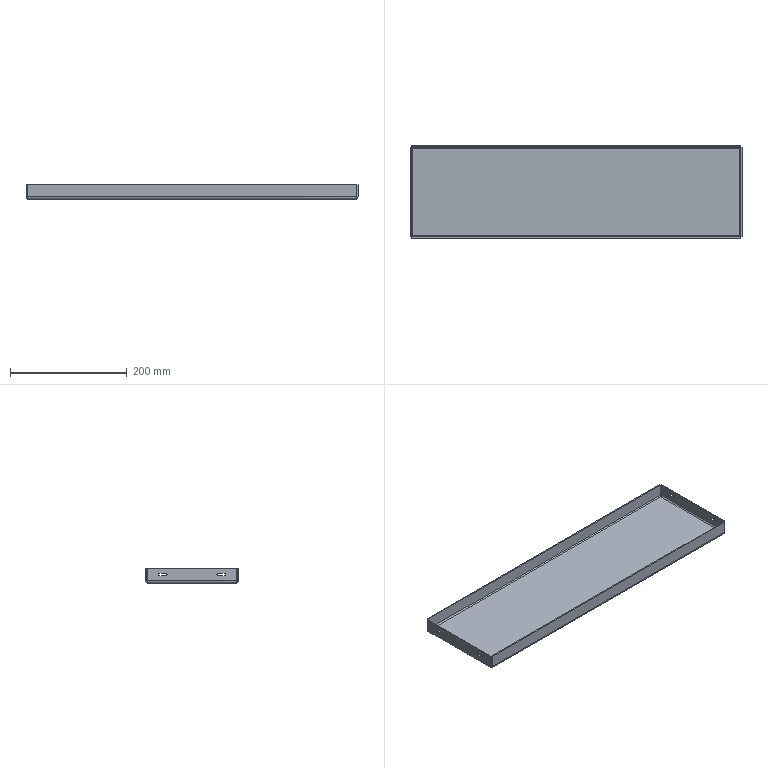Part | SolidWorks | features EdgeFlange 1, FlatPattern 1, ICE 1, SMBaseFlange 1, SheetMetal 1 | 1 solid | 54 faces | box 568 x 158 x 25 mm | volume 241019 mm3 | plane 30 | cylinder 16 | spline 8 | commonest cylinder face diameters 4.5 x8 4 x4 8 x4